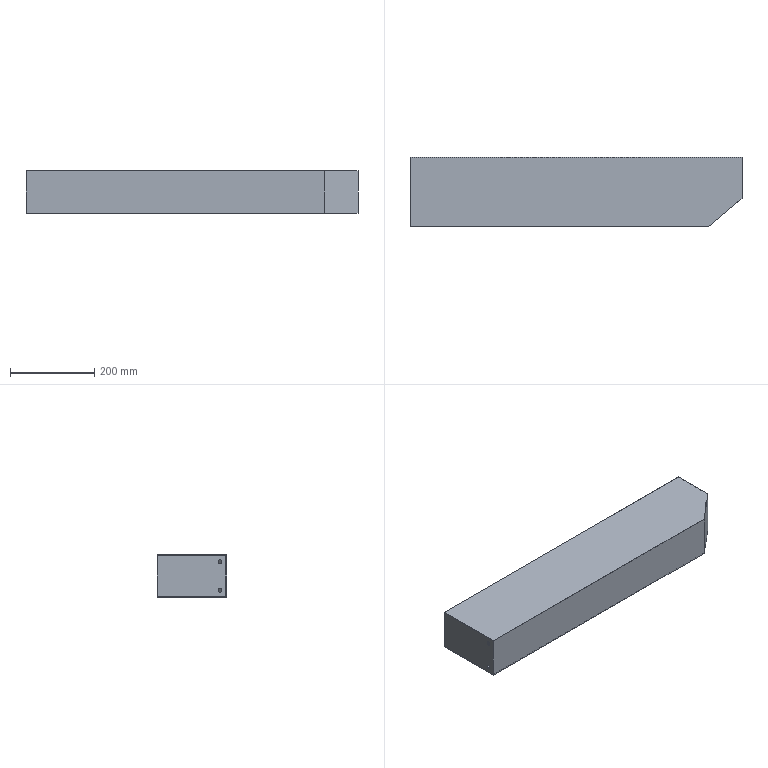Part | SolidWorks | features ICE 2, Extrusion 1, Shell 1 | 1 solid | 21 faces | box 787 x 165 x 100 mm | volume 713791 mm3 | plane 13 | cylinder 8 | commonest cylinder face diameters 9 x8
STEP:
#1=CARTESIAN_POINT('',(785.,83.,11.5));
#2=VERTEX_POINT('',#1);
#3=CARTESIAN_POINT('',(785.,83.,20.5));
#4=VERTEX_POINT('',#3);
#5=CARTESIAN_POINT('',(785.,83.,16.));
#6=DIRECTION('',(-1.,0.,0.));
#7=DIRECTION('',(0.,0.,1.));
#8=AXIS2_PLACEMENT_3D('',#5,#6,#7);
#9=CIRCLE('',#8,4.5);
#10=EDGE_CURVE('',#2,#4,#9,.T.);
#11=ORIENTED_EDGE('',*,*,#10,.T.);
#12=CARTESIAN_POINT('',(787.,83.,20.5));
#13=VERTEX_POINT('',#12);
#14=CARTESIAN_POINT('',(777.,83.,20.5));
#15=DIRECTION('',(1.,0.,0.));
#16=VECTOR('',#15,1000.);
#17=LINE('',#14,#16);
#18=EDGE_CURVE('',#4,#13,#17,.T.);
#19=ORIENTED_EDGE('',*,*,#18,.T.);
#20=CARTESIAN_POINT('',(787.,83.,11.5));
#21=VERTEX_POINT('',#20);
#22=CARTESIAN_POINT('',(787.,83.,16.));
#23=DIRECTION('',(1.,0.,0.));
#24=DIRECTION('',(0.,0.,-1.));
#25=AXIS2_PLACEMENT_3D('',#22,#23,#24);
#26=CIRCLE('',#25,4.5);
#27=EDGE_CURVE('',#13,#21,#26,.T.);
#28=ORIENTED_EDGE('',*,*,#27,.T.);
#29=CARTESIAN_POINT('',(777.,83.,11.5));
#30=DIRECTION('',(1.,0.,0.));
#31=VECTOR('',#30,1000.);
#32=LINE('',#29,#31);
#33=EDGE_CURVE('',#2,#21,#32,.T.);
#34=ORIENTED_EDGE('',*,*,#33,.F.);
#35=EDGE_LOOP('',(#11,#19,#28,#34));
#36=FACE_OUTER_BOUND('',#35,.T.);
#37=CARTESIAN_POINT('',(777.,83.,16.));
#38=DIRECTION('',(1.,0.,0.));
#39=DIRECTION('',(0.,0.,-1.));
#40=AXIS2_PLACEMENT_3D('',#37,#38,#39);
#41=CYLINDRICAL_SURFACE('',#40,4.5);
#42=ADVANCED_FACE('',(#36),#41,.F.);
#43=CARTESIAN_POINT('',(785.,83.,79.5));
#44=VERTEX_POINT('',#43);
#45=CARTESIAN_POINT('',(785.,83.,88.5));
#46=VERTEX_POINT('',#45);
#47=CARTESIAN_POINT('',(785.,83.,84.));
#48=DIRECTION('',(-1.,0.,0.));
#49=DIRECTION('',(0.,0.,1.));
#50=AXIS2_PLACEMENT_3D('',#47,#48,#49);
#51=CIRCLE('',#50,4.5);
#52=EDGE_CURVE('',#44,#46,#51,.T.);
#53=ORIENTED_EDGE('',*,*,#52,.T.);
#54=CARTESIAN_POINT('',(787.,83.,88.5));
#55=VERTEX_POINT('',#54);
#56=CARTESIAN_POINT('',(777.,83.,88.5));
#57=DIRECTION('',(1.,0.,0.));
#58=VECTOR('',#57,1000.);
#59=LINE('',#56,#58);
#60=EDGE_CURVE('',#46,#55,#59,.T.);
#61=ORIENTED_EDGE('',*,*,#60,.T.);
#62=CARTESIAN_POINT('',(787.,83.,79.5));
#63=VERTEX_POINT('',#62);
#64=CARTESIAN_POINT('',(787.,83.,84.));
#65=DIRECTION('',(1.,0.,0.));
#66=DIRECTION('',(0.,0.,-1.));
#67=AXIS2_PLACEMENT_3D('',#64,#65,#66);
#68=CIRCLE('',#67,4.5);
#69=EDGE_CURVE('',#55,#63,#68,.T.);
#70=ORIENTED_EDGE('',*,*,#69,.T.);
#71=CARTESIAN_POINT('',(777.,83.,79.5));
#72=DIRECTION('',(1.,0.,0.));
#73=VECTOR('',#72,1000.);
#74=LINE('',#71,#73);
#75=EDGE_CURVE('',#44,#63,#74,.T.);
#76=ORIENTED_EDGE('',*,*,#75,.F.);
#77=EDGE_LOOP('',(#53,#61,#70,#76));
#78=FACE_OUTER_BOUND('',#77,.T.);
#79=CARTESIAN_POINT('',(777.,83.,84.));
#80=DIRECTION('',(1.,0.,0.));
#81=DIRECTION('',(0.,0.,-1.));
#82=AXIS2_PLACEMENT_3D('',#79,#80,#81);
#83=CYLINDRICAL_SURFACE('',#82,4.5);
#84=ADVANCED_FACE('',(#78),#83,.F.);
#85=CARTESIAN_POINT('',(2.,11.5,84.));
#86=VERTEX_POINT('',#85);
#87=CARTESIAN_POINT('',(2.,20.5,84.));
#88=VERTEX_POINT('',#87);
#89=CARTESIAN_POINT('',(2.,16.,84.));
#90=DIRECTION('',(1.,0.,0.));
#91=DIRECTION('',(0.,1.,0.));
#92=AXIS2_PLACEMENT_3D('',#89,#90,#91);
#93=CIRCLE('',#92,4.5);
#94=EDGE_CURVE('',#86,#88,#93,.T.);
#95=ORIENTED_EDGE('',*,*,#94,.T.);
#96=CARTESIAN_POINT('',(0.,20.5,84.));
#97=VERTEX_POINT('',#96);
#98=CARTESIAN_POINT('',(10.,20.5,84.));
#99=DIRECTION('',(-1.,0.,0.));
#100=VECTOR('',#99,1000.);
#101=LINE('',#98,#100);
#102=EDGE_CURVE('',#88,#97,#101,.T.);
#103=ORIENTED_EDGE('',*,*,#102,.T.);
#104=CARTESIAN_POINT('',(0.,11.5,84.));
#105=VERTEX_POINT('',#104);
#106=CARTESIAN_POINT('',(0.,16.,84.));
#107=DIRECTION('',(-1.,0.,0.));
#108=DIRECTION('',(0.,-1.,0.));
#109=AXIS2_PLACEMENT_3D('',#106,#107,#108);
#110=CIRCLE('',#109,4.5);
#111=EDGE_CURVE('',#97,#105,#110,.T.);
#112=ORIENTED_EDGE('',*,*,#111,.T.);
#113=CARTESIAN_POINT('',(10.,11.5,84.));
#114=DIRECTION('',(-1.,0.,0.));
#115=VECTOR('',#114,1000.);
#116=LINE('',#113,#115);
#117=EDGE_CURVE('',#86,#105,#116,.T.);
#118=ORIENTED_EDGE('',*,*,#117,.F.);
#119=EDGE_LOOP('',(#95,#103,#112,#118));
#120=FACE_OUTER_BOUND('',#119,.T.);
#121=CARTESIAN_POINT('',(10.,16.,84.));
#122=DIRECTION('',(-1.,0.,0.));
#123=DIRECTION('',(0.,-1.,0.));
#124=AXIS2_PLACEMENT_3D('',#121,#122,#123);
#125=CYLINDRICAL_SURFACE('',#124,4.5);
#126=ADVANCED_FACE('',(#120),#125,.F.);
#127=CARTESIAN_POINT('',(2.,11.5,16.));
#128=VERTEX_POINT('',#127);
#129=CARTESIAN_POINT('',(2.,20.5,16.));
#130=VERTEX_POINT('',#129);
#131=CARTESIAN_POINT('',(2.,16.,16.));
#132=DIRECTION('',(1.,0.,0.));
#133=DIRECTION('',(0.,1.,0.));
#134=AXIS2_PLACEMENT_3D('',#131,#132,#133);
#135=CIRCLE('',#134,4.5);
#136=EDGE_CURVE('',#128,#130,#135,.T.);
#137=ORIENTED_EDGE('',*,*,#136,.T.);
#138=CARTESIAN_POINT('',(0.,20.5,16.));
#139=VERTEX_POINT('',#138);
#140=CARTESIAN_POINT('',(10.,20.5,16.));
#141=DIRECTION('',(-1.,0.,0.));
#142=VECTOR('',#141,1000.);
#143=LINE('',#140,#142);
#144=EDGE_CURVE('',#130,#139,#143,.T.);
#145=ORIENTED_EDGE('',*,*,#144,.T.);
#146=CARTESIAN_POINT('',(0.,11.5,16.));
#147=VERTEX_POINT('',#146);
#148=CARTESIAN_POINT('',(0.,16.,16.));
#149=DIRECTION('',(-1.,0.,0.));
#150=DIRECTION('',(0.,-1.,0.));
#151=AXIS2_PLACEMENT_3D('',#148,#149,#150);
#152=CIRCLE('',#151,4.5);
#153=EDGE_CURVE('',#139,#147,#152,.T.);
#154=ORIENTED_EDGE('',*,*,#153,.T.);
#155=CARTESIAN_POINT('',(10.,11.5,16.));
#156=DIRECTION('',(-1.,0.,0.));
#157=VECTOR('',#156,1000.);
#158=LINE('',#155,#157);
#159=EDGE_CURVE('',#128,#147,#158,.T.);
#160=ORIENTED_EDGE('',*,*,#159,.F.);
#161=EDGE_LOOP('',(#137,#145,#154,#160));
#162=FACE_OUTER_BOUND('',#161,.T.);
#163=CARTESIAN_POINT('',(10.,16.,16.));
#164=DIRECTION('',(-1.,0.,0.));
#165=DIRECTION('',(0.,-1.,0.));
#166=AXIS2_PLACEMENT_3D('',#163,#164,#165);
#167=CYLINDRICAL_SURFACE('',#166,4.5);
#168=ADVANCED_FACE('',(#162),#167,.F.);
#169=CARTESIAN_POINT('',(787.,165.,0.));
#170=VERTEX_POINT('',#169);
#171=CARTESIAN_POINT('',(0.,165.,0.));
#172=VERTEX_POINT('',#171);
#173=CARTESIAN_POINT('',(787.,165.,0.));
#174=DIRECTION('',(-1.,0.,0.));
#175=VECTOR('',#174,1000.);
#176=LINE('',#173,#175);
#177=EDGE_CURVE('',#170,#172,#176,.T.);
#178=ORIENTED_EDGE('',*,*,#177,.T.);
#179=CARTESIAN_POINT('',(0.,165.,100.));
#180=VERTEX_POINT('',#179);
#181=CARTESIAN_POINT('',(0.,165.,100.));
#182=DIRECTION('',(0.,0.,-1.));
#183=VECTOR('',#182,1000.);
#184=LINE('',#181,#183);
#185=EDGE_CURVE('',#180,#172,#184,.T.);
#186=ORIENTED_EDGE('',*,*,#185,.F.);
#187=CARTESIAN_POINT('',(787.,165.,100.));
#188=VERTEX_POINT('',#187);
#189=CARTESIAN_POINT('',(787.,165.,100.));
#190=DIRECTION('',(-1.,0.,0.));
#191=VECTOR('',#190,1000.);
#192=LINE('',#189,#191);
#193=EDGE_CURVE('',#188,#180,#192,.T.);
#194=ORIENTED_EDGE('',*,*,#193,.F.);
#195=CARTESIAN_POINT('',(787.,165.,100.));
#196=DIRECTION('',(0.,0.,-1.));
#197=VECTOR('',#196,1000.);
#198=LINE('',#195,#197);
#199=EDGE_CURVE('',#188,#170,#198,.T.);
#200=ORIENTED_EDGE('',*,*,#199,.T.);
#201=EDGE_LOOP('',(#178,#186,#194,#200));
#202=FACE_OUTER_BOUND('',#201,.T.);
#203=CARTESIAN_POINT('',(785.,165.,2.));
#204=VERTEX_POINT('',#203);
#205=CARTESIAN_POINT('',(2.,165.,2.));
#206=VERTEX_POINT('',#205);
#207=CARTESIAN_POINT('',(787.,165.,2.));
#208=DIRECTION('',(-1.,0.,0.));
#209=VECTOR('',#208,1000.);
#210=LINE('',#207,#209);
#211=EDGE_CURVE('',#204,#206,#210,.T.);
#212=ORIENTED_EDGE('',*,*,#211,.F.);
#213=CARTESIAN_POINT('',(785.,165.,98.));
#214=VERTEX_POINT('',#213);
#215=CARTESIAN_POINT('',(785.,165.,100.));
#216=DIRECTION('',(0.,0.,-1.));
#217=VECTOR('',#216,1000.);
#218=LINE('',#215,#217);
#219=EDGE_CURVE('',#214,#204,#218,.T.);
#220=ORIENTED_EDGE('',*,*,#219,.F.);
#221=CARTESIAN_POINT('',(2.,165.,98.));
#222=VERTEX_POINT('',#221);
#223=CARTESIAN_POINT('',(787.,165.,98.));
#224=DIRECTION('',(-1.,0.,0.));
#225=VECTOR('',#224,1000.);
#226=LINE('',#223,#225);
#227=EDGE_CURVE('',#214,#222,#226,.T.);
#228=ORIENTED_EDGE('',*,*,#227,.T.);
#229=CARTESIAN_POINT('',(2.,165.,100.));
#230=DIRECTION('',(0.,0.,-1.));
#231=VECTOR('',#230,1000.);
#232=LINE('',#229,#231);
#233=EDGE_CURVE('',#222,#206,#232,.T.);
#234=ORIENTED_EDGE('',*,*,#233,.T.);
#235=EDGE_LOOP('',(#212,#220,#228,#234));
#236=FACE_BOUND('',#235,.T.);
#237=CARTESIAN_POINT('',(787.,165.,100.));
#238=DIRECTION('',(0.,-1.,0.));
#239=DIRECTION('',(1.,0.,0.));
#240=AXIS2_PLACEMENT_3D('',#237,#238,#239);
#241=PLANE('',#240);
#242=ADVANCED_FACE('',(#202,#236),#241,.F.);
#243=CARTESIAN_POINT('',(0.,16.,84.));
#244=DIRECTION('',(-1.,0.,0.));
#245=DIRECTION('',(0.,-1.,0.));
#246=AXIS2_PLACEMENT_3D('',#243,#244,#245);
#247=CIRCLE('',#246,4.5);
#248=EDGE_CURVE('',#105,#97,#247,.T.);
#249=ORIENTED_EDGE('',*,*,#248,.F.);
#250=ORIENTED_EDGE('',*,*,#111,.F.);
#251=EDGE_LOOP('',(#249,#250));
#252=FACE_BOUND('',#251,.T.);
#253=CARTESIAN_POINT('',(0.,16.,16.));
#254=DIRECTION('',(-1.,0.,0.));
#255=DIRECTION('',(0.,-1.,0.));
#256=AXIS2_PLACEMENT_3D('',#253,#254,#255);
#257=CIRCLE('',#256,4.5);
#258=EDGE_CURVE('',#147,#139,#257,.T.);
#259=ORIENTED_EDGE('',*,*,#258,.F.);
#260=ORIENTED_EDGE('',*,*,#153,.F.);
#261=EDGE_LOOP('',(#259,#260));
#262=FACE_BOUND('',#261,.T.);
#263=CARTESIAN_POINT('',(0.,0.,0.));
#264=VERTEX_POINT('',#263);
#265=CARTESIAN_POINT('',(0.,165.,0.));
#266=DIRECTION('',(0.,-1.,0.));
#267=VECTOR('',#266,1000.);
#268=LINE('',#265,#267);
#269=EDGE_CURVE('',#172,#264,#268,.T.);
#270=ORIENTED_EDGE('',*,*,#269,.T.);
#271=CARTESIAN_POINT('',(0.,0.,100.));
#272=VERTEX_POINT('',#271);
#273=CARTESIAN_POINT('',(0.,0.,100.));
#274=DIRECTION('',(0.,0.,-1.));
#275=VECTOR('',#274,1000.);
#276=LINE('',#273,#275);
#277=EDGE_CURVE('',#272,#264,#276,.T.);
#278=ORIENTED_EDGE('',*,*,#277,.F.);
#279=CARTESIAN_POINT('',(0.,165.,100.));
#280=DIRECTION('',(0.,-1.,0.));
#281=VECTOR('',#280,1000.);
#282=LINE('',#279,#281);
#283=EDGE_CURVE('',#180,#272,#282,.T.);
#284=ORIENTED_EDGE('',*,*,#283,.F.);
#285=ORIENTED_EDGE('',*,*,#185,.T.);
#286=EDGE_LOOP('',(#270,#278,#284,#285));
#287=FACE_OUTER_BOUND('',#286,.T.);
#288=CARTESIAN_POINT('',(0.,165.,100.));
#289=DIRECTION('',(1.,0.,0.));
#290=DIRECTION('',(0.,1.,0.));
#291=AXIS2_PLACEMENT_3D('',#288,#289,#290);
#292=PLANE('',#291);
#293=ADVANCED_FACE('',(#252,#262,#287),#292,.F.);
#294=CARTESIAN_POINT('',(707.153,0.,0.));
#295=VERTEX_POINT('',#294);
#296=CARTESIAN_POINT('',(0.,0.,0.));
#297=DIRECTION('',(1.,0.,0.));
#298=VECTOR('',#297,1000.);
#299=LINE('',#296,#298);
#300=EDGE_CURVE('',#264,#295,#299,.T.);
#301=ORIENTED_EDGE('',*,*,#300,.T.);
#302=CARTESIAN_POINT('',(707.153,0.,100.));
#303=VERTEX_POINT('',#302);
#304=CARTESIAN_POINT('',(707.153,0.,100.));
#305=DIRECTION('',(0.,0.,-1.));
#306=VECTOR('',#305,1000.);
#307=LINE('',#304,#306);
#308=EDGE_CURVE('',#303,#295,#307,.T.);
#309=ORIENTED_EDGE('',*,*,#308,.F.);
#310=CARTESIAN_POINT('',(0.,0.,100.));
#311=DIRECTION('',(1.,0.,0.));
#312=VECTOR('',#311,1000.);
#313=LINE('',#310,#312);
#314=EDGE_CURVE('',#272,#303,#313,.T.);
#315=ORIENTED_EDGE('',*,*,#314,.F.);
#316=ORIENTED_EDGE('',*,*,#277,.T.);
#317=EDGE_LOOP('',(#301,#309,#315,#316));
#318=FACE_OUTER_BOUND('',#317,.T.);
#319=CARTESIAN_POINT('',(0.,0.,100.));
#320=DIRECTION('',(0.,1.,0.));
#321=DIRECTION('',(0.,0.,1.));
#322=AXIS2_PLACEMENT_3D('',#319,#320,#321);
#323=PLANE('',#322);
#324=ADVANCED_FACE('',(#318),#323,.F.);
#325=CARTESIAN_POINT('',(787.,67.,0.));
#326=VERTEX_POINT('',#325);
#327=CARTESIAN_POINT('',(707.153,0.,0.));
#328=DIRECTION('',(0.766,0.6428,0.));
#329=VECTOR('',#328,1000.);
#330=LINE('',#327,#329);
#331=EDGE_CURVE('',#295,#326,#330,.T.);
#332=ORIENTED_EDGE('',*,*,#331,.T.);
#333=CARTESIAN_POINT('',(787.,67.,100.));
#334=VERTEX_POINT('',#333);
#335=CARTESIAN_POINT('',(787.,67.,100.));
#336=DIRECTION('',(0.,0.,-1.));
#337=VECTOR('',#336,1000.);
#338=LINE('',#335,#337);
#339=EDGE_CURVE('',#334,#326,#338,.T.);
#340=ORIENTED_EDGE('',*,*,#339,.F.);
#341=CARTESIAN_POINT('',(707.153,0.,100.));
#342=DIRECTION('',(0.766,0.6428,0.));
#343=VECTOR('',#342,1000.);
#344=LINE('',#341,#343);
#345=EDGE_CURVE('',#303,#334,#344,.T.);
#346=ORIENTED_EDGE('',*,*,#345,.F.);
#347=ORIENTED_EDGE('',*,*,#308,.T.);
#348=EDGE_LOOP('',(#332,#340,#346,#347));
#349=FACE_OUTER_BOUND('',#348,.T.);
#350=CARTESIAN_POINT('',(707.153,0.,100.));
#351=DIRECTION('',(-0.6428,0.766,0.));
#352=DIRECTION('',(-0.766,-0.6428,0.));
#353=AXIS2_PLACEMENT_3D('',#350,#351,#352);
#354=PLANE('',#353);
#355=ADVANCED_FACE('',(#349),#354,.F.);
#356=CARTESIAN_POINT('',(787.,83.,16.));
#357=DIRECTION('',(1.,0.,0.));
#358=DIRECTION('',(0.,0.,-1.));
#359=AXIS2_PLACEMENT_3D('',#356,#357,#358);
#360=CIRCLE('',#359,4.5);
#361=EDGE_CURVE('',#21,#13,#360,.T.);
#362=ORIENTED_EDGE('',*,*,#361,.F.);
#363=ORIENTED_EDGE('',*,*,#27,.F.);
#364=EDGE_LOOP('',(#362,#363));
#365=FACE_BOUND('',#364,.T.);
#366=CARTESIAN_POINT('',(787.,83.,84.));
#367=DIRECTION('',(1.,0.,0.));
#368=DIRECTION('',(0.,0.,-1.));
#369=AXIS2_PLACEMENT_3D('',#366,#367,#368);
#370=CIRCLE('',#369,4.5);
#371=EDGE_CURVE('',#63,#55,#370,.T.);
#372=ORIENTED_EDGE('',*,*,#371,.F.);
#373=ORIENTED_EDGE('',*,*,#69,.F.);
#374=EDGE_LOOP('',(#372,#373));
#375=FACE_BOUND('',#374,.T.);
#376=CARTESIAN_POINT('',(787.,67.,0.));
#377=DIRECTION('',(0.,1.,0.));
#378=VECTOR('',#377,1000.);
#379=LINE('',#376,#378);
#380=EDGE_CURVE('',#326,#170,#379,.T.);
#381=ORIENTED_EDGE('',*,*,#380,.T.);
#382=ORIENTED_EDGE('',*,*,#199,.F.);
#383=CARTESIAN_POINT('',(787.,67.,100.));
#384=DIRECTION('',(0.,1.,0.));
#385=VECTOR('',#384,1000.);
#386=LINE('',#383,#385);
#387=EDGE_CURVE('',#334,#188,#386,.T.);
#388=ORIENTED_EDGE('',*,*,#387,.F.);
#389=ORIENTED_EDGE('',*,*,#339,.T.);
#390=EDGE_LOOP('',(#381,#382,#388,#389));
#391=FACE_OUTER_BOUND('',#390,.T.);
#392=CARTESIAN_POINT('',(787.,67.,100.));
#393=DIRECTION('',(-1.,0.,0.));
#394=DIRECTION('',(0.,0.,1.));
#395=AXIS2_PLACEMENT_3D('',#392,#393,#394);
#396=PLANE('',#395);
#397=ADVANCED_FACE('',(#365,#375,#391),#396,.F.);
#398=ORIENTED_EDGE('',*,*,#283,.T.);
#399=ORIENTED_EDGE('',*,*,#314,.T.);
#400=ORIENTED_EDGE('',*,*,#345,.T.);
#401=ORIENTED_EDGE('',*,*,#387,.T.);
#402=ORIENTED_EDGE('',*,*,#193,.T.);
#403=EDGE_LOOP('',(#398,#399,#400,#401,#402));
#404=FACE_OUTER_BOUND('',#403,.T.);
#405=CARTESIAN_POINT('',(0.,0.,100.));
#406=DIRECTION('',(0.,0.,1.));
#407=DIRECTION('',(1.,0.,0.));
#408=AXIS2_PLACEMENT_3D('',#405,#406,#407);
#409=PLANE('',#408);
#410=ADVANCED_FACE('',(#404),#409,.T.);
#411=ORIENTED_EDGE('',*,*,#269,.F.);
#412=ORIENTED_EDGE('',*,*,#177,.F.);
#413=ORIENTED_EDGE('',*,*,#380,.F.);
#414=ORIENTED_EDGE('',*,*,#331,.F.);
#415=ORIENTED_EDGE('',*,*,#300,.F.);
#416=EDGE_LOOP('',(#411,#412,#413,#414,#415));
#417=FACE_OUTER_BOUND('',#416,.T.);
#418=CARTESIAN_POINT('',(0.,0.,0.));
#419=DIRECTION('',(0.,0.,1.));
#420=DIRECTION('',(1.,0.,0.));
#421=AXIS2_PLACEMENT_3D('',#418,#419,#420);
#422=PLANE('',#421);
#423=ADVANCED_FACE('',(#417),#422,.F.);
#424=ORIENTED_EDGE('',*,*,#94,.F.);
#425=CARTESIAN_POINT('',(2.,16.,84.));
#426=DIRECTION('',(1.,0.,0.));
#427=DIRECTION('',(0.,1.,0.));
#428=AXIS2_PLACEMENT_3D('',#425,#426,#427);
#429=CIRCLE('',#428,4.5);
#430=EDGE_CURVE('',#88,#86,#429,.T.);
#431=ORIENTED_EDGE('',*,*,#430,.F.);
#432=EDGE_LOOP('',(#424,#431));
#433=FACE_BOUND('',#432,.T.);
#434=ORIENTED_EDGE('',*,*,#136,.F.);
#435=CARTESIAN_POINT('',(2.,16.,16.));
#436=DIRECTION('',(1.,0.,0.));
#437=DIRECTION('',(0.,1.,0.));
#438=AXIS2_PLACEMENT_3D('',#435,#436,#437);
#439=CIRCLE('',#438,4.5);
#440=EDGE_CURVE('',#130,#128,#439,.T.);
#441=ORIENTED_EDGE('',*,*,#440,.F.);
#442=EDGE_LOOP('',(#434,#441));
#443=FACE_BOUND('',#442,.T.);
#444=CARTESIAN_POINT('',(2.,2.,2.));
#445=VERTEX_POINT('',#444);
#446=CARTESIAN_POINT('',(2.,165.,2.));
#447=DIRECTION('',(0.,-1.,0.));
#448=VECTOR('',#447,1000.);
#449=LINE('',#446,#448);
#450=EDGE_CURVE('',#206,#445,#449,.T.);
#451=ORIENTED_EDGE('',*,*,#450,.F.);
#452=ORIENTED_EDGE('',*,*,#233,.F.);
#453=CARTESIAN_POINT('',(2.,2.,98.));
#454=VERTEX_POINT('',#453);
#455=CARTESIAN_POINT('',(2.,165.,98.));
#456=DIRECTION('',(0.,-1.,0.));
#457=VECTOR('',#456,1000.);
#458=LINE('',#455,#457);
#459=EDGE_CURVE('',#222,#454,#458,.T.);
#460=ORIENTED_EDGE('',*,*,#459,.T.);
#461=CARTESIAN_POINT('',(2.,2.,100.));
#462=DIRECTION('',(0.,0.,-1.));
#463=VECTOR('',#462,1000.);
#464=LINE('',#461,#463);
#465=EDGE_CURVE('',#454,#445,#464,.T.);
#466=ORIENTED_EDGE('',*,*,#465,.T.);
#467=EDGE_LOOP('',(#451,#452,#460,#466));
#468=FACE_OUTER_BOUND('',#467,.T.);
#469=CARTESIAN_POINT('',(2.,165.,100.));
#470=DIRECTION('',(1.,0.,0.));
#471=DIRECTION('',(0.,1.,0.));
#472=AXIS2_PLACEMENT_3D('',#469,#470,#471);
#473=PLANE('',#472);
#474=ADVANCED_FACE('',(#433,#443,#468),#473,.T.);
#475=CARTESIAN_POINT('',(706.425,2.,2.));
#476=VERTEX_POINT('',#475);
#477=CARTESIAN_POINT('',(0.,2.,2.));
#478=DIRECTION('',(1.,0.,0.));
#479=VECTOR('',#478,1000.);
#480=LINE('',#477,#479);
#481=EDGE_CURVE('',#445,#476,#480,.T.);
#482=ORIENTED_EDGE('',*,*,#481,.F.);
#483=ORIENTED_EDGE('',*,*,#465,.F.);
#484=CARTESIAN_POINT('',(706.425,2.,98.));
#485=VERTEX_POINT('',#484);
#486=CARTESIAN_POINT('',(0.,2.,98.));
#487=DIRECTION('',(1.,0.,0.));
#488=VECTOR('',#487,1000.);
#489=LINE('',#486,#488);
#490=EDGE_CURVE('',#454,#485,#489,.T.);
#491=ORIENTED_EDGE('',*,*,#490,.T.);
#492=CARTESIAN_POINT('',(706.425,2.,100.));
#493=DIRECTION('',(0.,0.,-1.));
#494=VECTOR('',#493,1000.);
#495=LINE('',#492,#494);
#496=EDGE_CURVE('',#485,#476,#495,.T.);
#497=ORIENTED_EDGE('',*,*,#496,.T.);
#498=EDGE_LOOP('',(#482,#483,#491,#497));
#499=FACE_OUTER_BOUND('',#498,.T.);
#500=CARTESIAN_POINT('',(0.,2.,100.));
#501=DIRECTION('',(0.,1.,0.));
#502=DIRECTION('',(0.,0.,1.));
#503=AXIS2_PLACEMENT_3D('',#500,#501,#502);
#504=PLANE('',#503);
#505=ADVANCED_FACE('',(#499),#504,.T.);
#506=CARTESIAN_POINT('',(785.,67.933,2.));
#507=VERTEX_POINT('',#506);
#508=CARTESIAN_POINT('',(705.867,1.532,2.));
#509=DIRECTION('',(0.766,0.6428,0.));
#510=VECTOR('',#509,1000.);
#511=LINE('',#508,#510);
#512=EDGE_CURVE('',#476,#507,#511,.T.);
#513=ORIENTED_EDGE('',*,*,#512,.F.);
#514=ORIENTED_EDGE('',*,*,#496,.F.);
#515=CARTESIAN_POINT('',(785.,67.933,98.));
#516=VERTEX_POINT('',#515);
#517=CARTESIAN_POINT('',(705.867,1.532,98.));
#518=DIRECTION('',(0.766,0.6428,0.));
#519=VECTOR('',#518,1000.);
#520=LINE('',#517,#519);
#521=EDGE_CURVE('',#485,#516,#520,.T.);
#522=ORIENTED_EDGE('',*,*,#521,.T.);
#523=CARTESIAN_POINT('',(785.,67.933,100.));
#524=DIRECTION('',(0.,0.,-1.));
#525=VECTOR('',#524,1000.);
#526=LINE('',#523,#525);
#527=EDGE_CURVE('',#516,#507,#526,.T.);
#528=ORIENTED_EDGE('',*,*,#527,.T.);
#529=EDGE_LOOP('',(#513,#514,#522,#528));
#530=FACE_OUTER_BOUND('',#529,.T.);
#531=CARTESIAN_POINT('',(705.867,1.532,100.));
#532=DIRECTION('',(-0.6428,0.766,0.));
#533=DIRECTION('',(-0.766,-0.6428,0.));
#534=AXIS2_PLACEMENT_3D('',#531,#532,#533);
#535=PLANE('',#534);
#536=ADVANCED_FACE('',(#530),#535,.T.);
#537=ORIENTED_EDGE('',*,*,#10,.F.);
#538=CARTESIAN_POINT('',(785.,83.,16.));
#539=DIRECTION('',(-1.,0.,0.));
#540=DIRECTION('',(0.,0.,1.));
#541=AXIS2_PLACEMENT_3D('',#538,#539,#540);
#542=CIRCLE('',#541,4.5);
#543=EDGE_CURVE('',#4,#2,#542,.T.);
#544=ORIENTED_EDGE('',*,*,#543,.F.);
#545=EDGE_LOOP('',(#537,#544));
#546=FACE_BOUND('',#545,.T.);
#547=ORIENTED_EDGE('',*,*,#52,.F.);
#548=CARTESIAN_POINT('',(785.,83.,84.));
#549=DIRECTION('',(-1.,0.,0.));
#550=DIRECTION('',(0.,0.,1.));
#551=AXIS2_PLACEMENT_3D('',#548,#549,#550);
#552=CIRCLE('',#551,4.5);
#553=EDGE_CURVE('',#46,#44,#552,.T.);
#554=ORIENTED_EDGE('',*,*,#553,.F.);
#555=EDGE_LOOP('',(#547,#554));
#556=FACE_BOUND('',#555,.T.);
#557=CARTESIAN_POINT('',(785.,67.,2.));
#558=DIRECTION('',(0.,1.,0.));
#559=VECTOR('',#558,1000.);
#560=LINE('',#557,#559);
#561=EDGE_CURVE('',#507,#204,#560,.T.);
#562=ORIENTED_EDGE('',*,*,#561,.F.);
#563=ORIENTED_EDGE('',*,*,#527,.F.);
#564=CARTESIAN_POINT('',(785.,67.,98.));
#565=DIRECTION('',(0.,1.,0.));
#566=VECTOR('',#565,1000.);
#567=LINE('',#564,#566);
#568=EDGE_CURVE('',#516,#214,#567,.T.);
#569=ORIENTED_EDGE('',*,*,#568,.T.);
#570=ORIENTED_EDGE('',*,*,#219,.T.);
#571=EDGE_LOOP('',(#562,#563,#569,#570));
#572=FACE_OUTER_BOUND('',#571,.T.);
#573=CARTESIAN_POINT('',(785.,67.,100.));
#574=DIRECTION('',(-1.,0.,0.));
#575=DIRECTION('',(0.,0.,1.));
#576=AXIS2_PLACEMENT_3D('',#573,#574,#575);
#577=PLANE('',#576);
#578=ADVANCED_FACE('',(#546,#556,#572),#577,.T.);
#579=ORIENTED_EDGE('',*,*,#459,.F.);
#580=ORIENTED_EDGE('',*,*,#227,.F.);
#581=ORIENTED_EDGE('',*,*,#568,.F.);
#582=ORIENTED_EDGE('',*,*,#521,.F.);
#583=ORIENTED_EDGE('',*,*,#490,.F.);
#584=EDGE_LOOP('',(#579,#580,#581,#582,#583));
#585=FACE_OUTER_BOUND('',#584,.T.);
#586=CARTESIAN_POINT('',(0.,0.,98.));
#587=DIRECTION('',(0.,0.,1.));
#588=DIRECTION('',(1.,0.,0.));
#589=AXIS2_PLACEMENT_3D('',#586,#587,#588);
#590=PLANE('',#589);
#591=ADVANCED_FACE('',(#585),#590,.F.);
#592=ORIENTED_EDGE('',*,*,#450,.T.);
#593=ORIENTED_EDGE('',*,*,#481,.T.);
#594=ORIENTED_EDGE('',*,*,#512,.T.);
#595=ORIENTED_EDGE('',*,*,#561,.T.);
#596=ORIENTED_EDGE('',*,*,#211,.T.);
#597=EDGE_LOOP('',(#592,#593,#594,#595,#596));
#598=FACE_OUTER_BOUND('',#597,.T.);
#599=CARTESIAN_POINT('',(0.,0.,2.));
#600=DIRECTION('',(0.,0.,1.));
#601=DIRECTION('',(1.,0.,0.));
#602=AXIS2_PLACEMENT_3D('',#599,#600,#601);
#603=PLANE('',#602);
#604=ADVANCED_FACE('',(#598),#603,.T.);
#605=ORIENTED_EDGE('',*,*,#144,.F.);
#606=ORIENTED_EDGE('',*,*,#440,.T.);
#607=ORIENTED_EDGE('',*,*,#159,.T.);
#608=ORIENTED_EDGE('',*,*,#258,.T.);
#609=EDGE_LOOP('',(#605,#606,#607,#608));
#610=FACE_OUTER_BOUND('',#609,.T.);
#611=CARTESIAN_POINT('',(10.,16.,16.));
#612=DIRECTION('',(-1.,0.,0.));
#613=DIRECTION('',(0.,-1.,0.));
#614=AXIS2_PLACEMENT_3D('',#611,#612,#613);
#615=CYLINDRICAL_SURFACE('',#614,4.5);
#616=ADVANCED_FACE('',(#610),#615,.F.);
#617=ORIENTED_EDGE('',*,*,#102,.F.);
#618=ORIENTED_EDGE('',*,*,#430,.T.);
#619=ORIENTED_EDGE('',*,*,#117,.T.);
#620=ORIENTED_EDGE('',*,*,#248,.T.);
#621=EDGE_LOOP('',(#617,#618,#619,#620));
#622=FACE_OUTER_BOUND('',#621,.T.);
#623=CARTESIAN_POINT('',(10.,16.,84.));
#624=DIRECTION('',(-1.,0.,0.));
#625=DIRECTION('',(0.,-1.,0.));
#626=AXIS2_PLACEMENT_3D('',#623,#624,#625);
#627=CYLINDRICAL_SURFACE('',#626,4.5);
#628=ADVANCED_FACE('',(#622),#627,.F.);
#629=ORIENTED_EDGE('',*,*,#60,.F.);
#630=ORIENTED_EDGE('',*,*,#553,.T.);
#631=ORIENTED_EDGE('',*,*,#75,.T.);
#632=ORIENTED_EDGE('',*,*,#371,.T.);
#633=EDGE_LOOP('',(#629,#630,#631,#632));
#634=FACE_OUTER_BOUND('',#633,.T.);
#635=CARTESIAN_POINT('',(777.,83.,84.));
#636=DIRECTION('',(1.,0.,0.));
#637=DIRECTION('',(0.,0.,-1.));
#638=AXIS2_PLACEMENT_3D('',#635,#636,#637);
#639=CYLINDRICAL_SURFACE('',#638,4.5);
#640=ADVANCED_FACE('',(#634),#639,.F.);
#641=ORIENTED_EDGE('',*,*,#18,.F.);
#642=ORIENTED_EDGE('',*,*,#543,.T.);
#643=ORIENTED_EDGE('',*,*,#33,.T.);
#644=ORIENTED_EDGE('',*,*,#361,.T.);
#645=EDGE_LOOP('',(#641,#642,#643,#644));
#646=FACE_OUTER_BOUND('',#645,.T.);
#647=CARTESIAN_POINT('',(777.,83.,16.));
#648=DIRECTION('',(1.,0.,0.));
#649=DIRECTION('',(0.,0.,-1.));
#650=AXIS2_PLACEMENT_3D('',#647,#648,#649);
#651=CYLINDRICAL_SURFACE('',#650,4.5);
#652=ADVANCED_FACE('',(#646),#651,.F.);
#653=CLOSED_SHELL('',(#42,#84,#126,#168,#242,#293,#324,#355,#397,#410,#423,#474,#505,#536,#578,#591,#604,#616,#628,#640,#652));
#654=MANIFOLD_SOLID_BREP('',#653);
#655=CARTESIAN_POINT('',(0.,0.,0.));
#656=DIRECTION('',(0.,0.,1.));
#657=DIRECTION('',(1.,0.,0.));
#658=AXIS2_PLACEMENT_3D('',#655,#656,#657);
#659=(LENGTH_UNIT()NAMED_UNIT(*)SI_UNIT(.MILLI.,.METRE.));
#660=UNCERTAINTY_MEASURE_WITH_UNIT(LENGTH_MEASURE(0.00001),#659,'','');
#661=(NAMED_UNIT(*)PLANE_ANGLE_UNIT()SI_UNIT($,.RADIAN.));
#662=(NAMED_UNIT(*)SI_UNIT($,.STERADIAN.)SOLID_ANGLE_UNIT());
#663=(GEOMETRIC_REPRESENTATION_CONTEXT(3)GLOBAL_UNCERTAINTY_ASSIGNED_CONTEXT((#660))GLOBAL_UNIT_ASSIGNED_CONTEXT((#659,#661,#662))REPRESENTATION_CONTEXT('',''));
#664=ADVANCED_BREP_SHAPE_REPRESENTATION('',(#654,#658),#663);